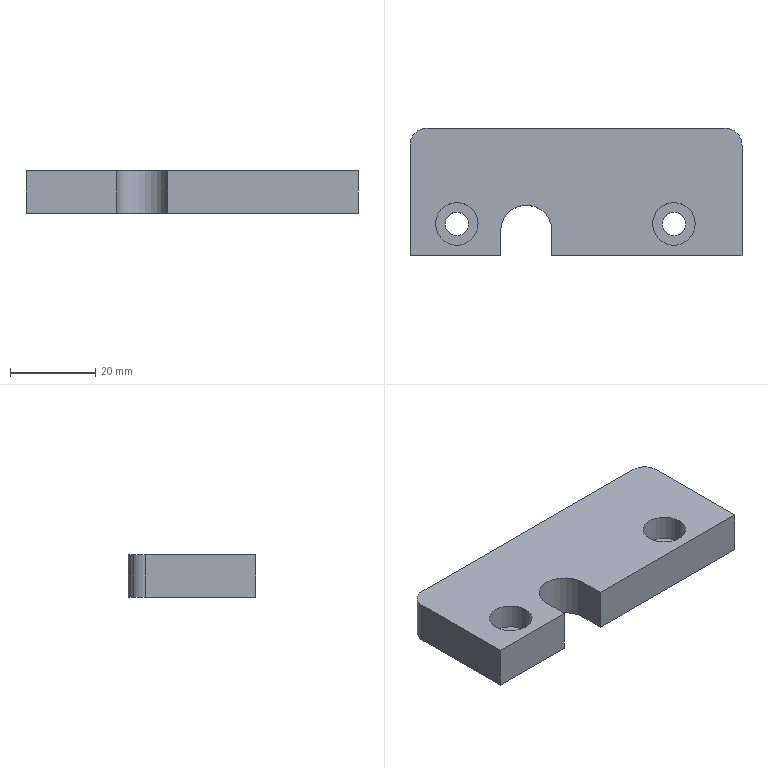Part | STEP file | ASND-0110-TCTF01-57 | 1 solid | 24 faces | box 78 x 30 x 10 mm | volume 20925 mm3 | cylinder 13 | plane 11 | commonest cylinder face diameters 5.5 x4 8 x4 10 x4 12 x1